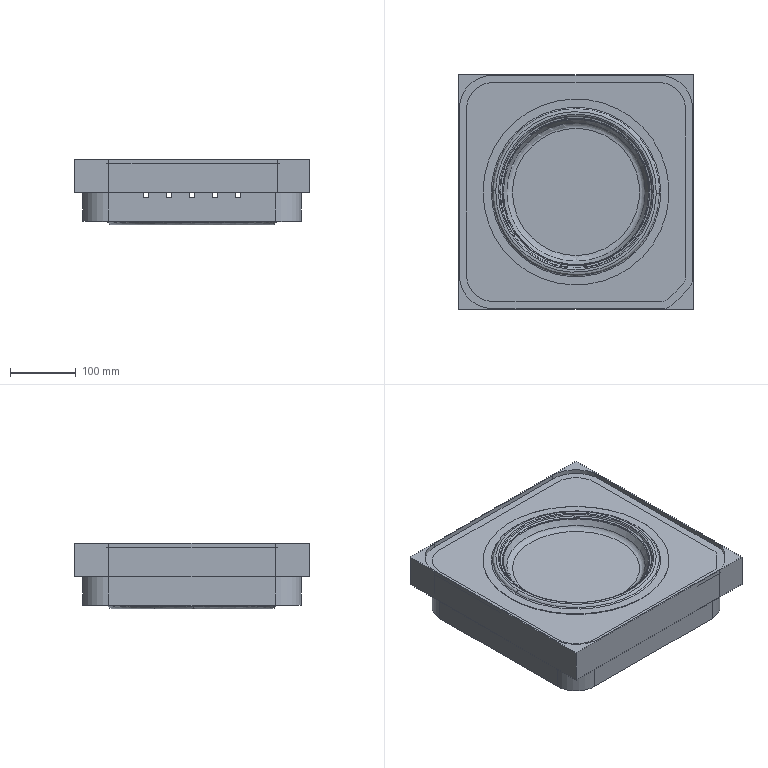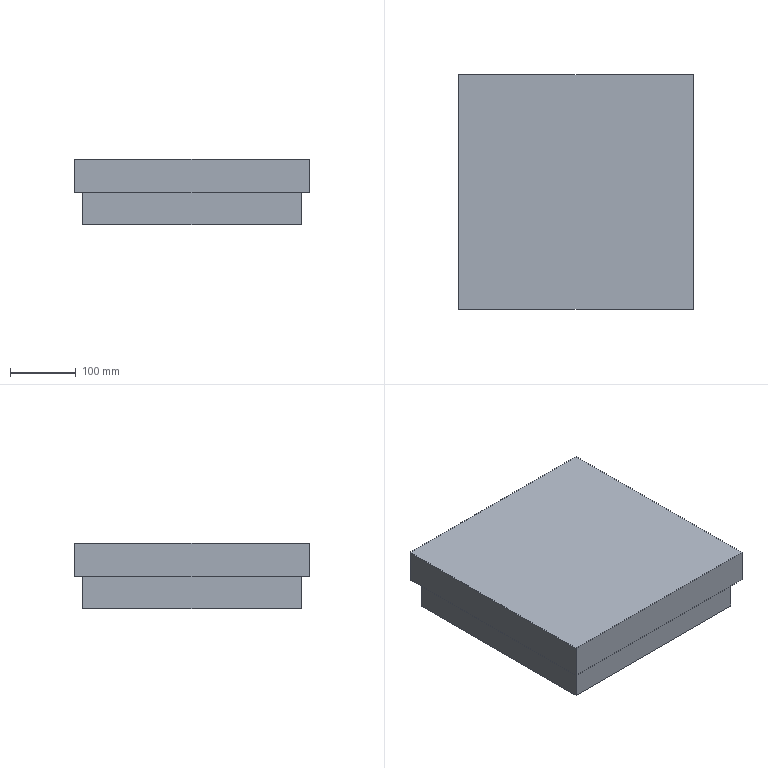CAM job | NX | 3-axis milling, drilling | part box 356 x 356 x 99.5 mm | stock box 356 x 356 x 99.5 mm
Tools:
number,name,description,diameter,corner_radius,flute_length,length,flutes
0,V2.0,Drilling Tool,2.0,0.0,35.0,50.0,2
0,V8.0,Drilling Tool,8.0,0.0,35.0,50.0,2
0,D10,No Description,10.0,0.0,20.0,60.0,2
0,D12,No Description,12.0,0.0,50.0,70.0,2
0,D8,No Description,8.0,0.0,0.0,40.0,2
0,D16R0.8,No Description,16.0,0.8,50.0,90.0,2
0,R2,No Description,4.0,2.0,0.0,20.0,2
Operations:
program,operation,operation_type,tool,method,geometry_group,spindle_rpm,surface_speed,feed_per_tooth,feed_cut,feed_plunge,cut_length_mm,path_length_mm,cut_time_min,machine_time_min
B-1,01,CavityMilling,D16R0.8,METHOD,22B,7000.0,1099.0,0.3214,4500.0,100.0,310214.176,316175.361,68.936,69.533
B-2,2,CavityMilling,D8,METHOD,22B,7000.0,1099.0,0.3214,4500.0,100.0,37400.408,38896.07,8.311,8.461
B-3,03,FaceMilling,D12,METHOD,22B,7000.0,1099.0,0.2857,4000.0,100.0,8545.395,8855.945,2.136,2.167
B-4,06,SurfaceContour,R2,METHOD,22B,8000.0,251.0,0.2812,4500.0,100.0,246272.953,246593.508,54.727,54.759
B-4,05,Engraving,R2,METHOD,22B,9000.0,113.0,0.1111,2000.0,100.0,975.874,9549.453,0.877,1.734
B-5,DRILLING,Operation,V2.0,METHOD,22B,2000.0,75.0,0.0375,150.0,0.0,435.0,3667.483,2.9,3.223
B-6,07,PlanarMilling,D10,METHOD,22B,7000.0,571.0,0.2857,4000.0,100.0,52311.945,52667.02,13.078,13.114
C-1,CAVITY_MILL_1,CavityMilling,D8,METHOD,23C,7000.0,1099.0,0.3214,4500.0,100.0,181802.492,183121.054,40.401,40.532
C-2,DRILLING_1,Operation,V2.0,METHOD,23C,2000.0,75.0,0.0375,150.0,0.0,165.0,1547.287,1.1,1.238
C-3,DRILLING_1_COPY,Operation,V8.0,METHOD,23C,2000.0,75.0,0.0375,150.0,0.0,660.0,2537.287,4.4,4.588